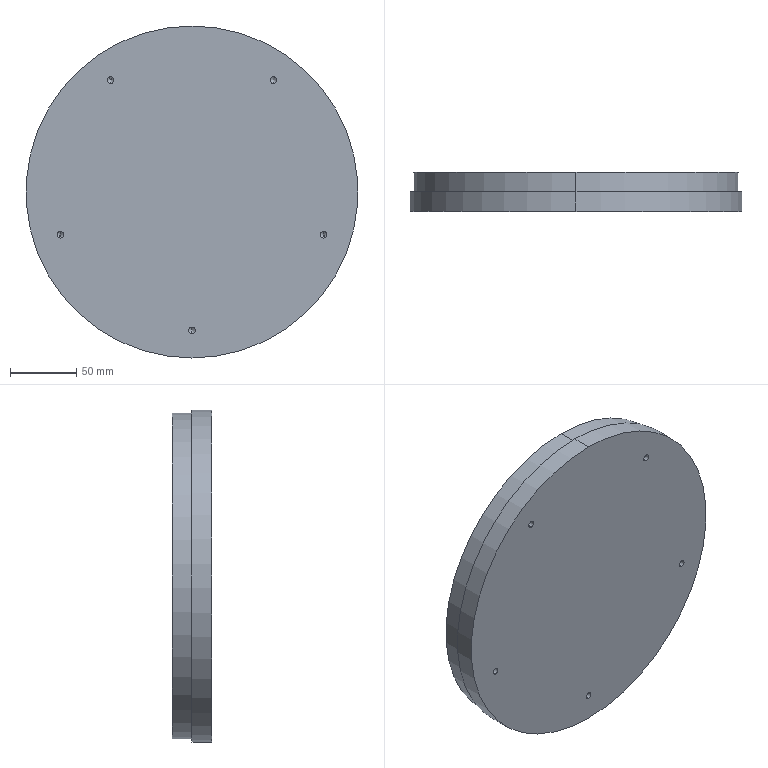Part | STEP file | 1 solid | 43 faces | box 249.9 x 29.4 x 249.9 mm | volume 1411943 mm3 | cylinder 22 | cone 18 | plane 3 | commonest cylinder face diameters 4.998 x10 4.165 x8 245 x2 249.9 x2